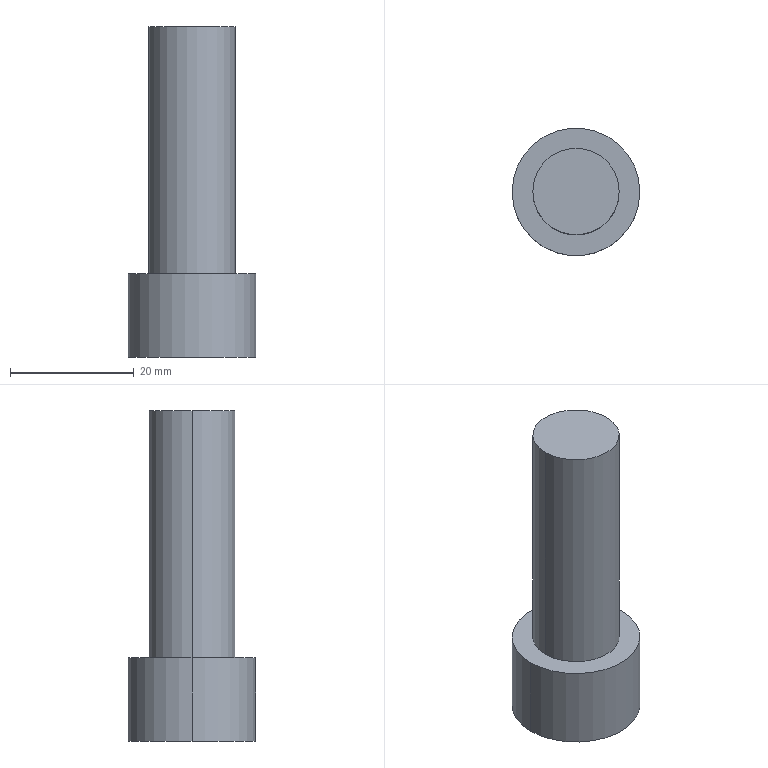Part | STEP file | M14 screw | 1 solid | 7 faces | box 20.67 x 20.67 x 53.57 mm | volume 10711 mm3 | cylinder 4 | plane 3 | commonest cylinder face diameters 14 x2 20.67 x2
STEP:
#1=CARTESIAN_POINT('',(0.,0.,0.));
#2=DIRECTION('',(0.,0.,1.));
#3=DIRECTION('',(1.,0.,0.));
#4=AXIS2_PLACEMENT_3D('',#1,#2,#3);
#5=CARTESIAN_POINT('',(7.,0.,53.57));
#6=VERTEX_POINT('',#5);
#7=CARTESIAN_POINT('',(-7.,0.,53.57));
#8=VERTEX_POINT('',#7);
#9=CARTESIAN_POINT('',(0.,0.,53.57));
#10=DIRECTION('',(0.,0.,1.));
#11=DIRECTION('',(1.,0.,0.));
#12=AXIS2_PLACEMENT_3D('',#9,#10,#11);
#13=CIRCLE('',#12,7.);
#14=CARTESIAN_POINT('',(0.,0.,53.57));
#15=DIRECTION('',(0.,0.,-1.));
#16=DIRECTION('',(-1.,0.,0.));
#17=AXIS2_PLACEMENT_3D('',#14,#15,#16);
#18=CYLINDRICAL_SURFACE('',#17,7.);
#19=CARTESIAN_POINT('',(3.142,0.));
#20=DIRECTION('',(-1.,0.));
#21=VECTOR('',#20,1.);
#22=LINE('',#19,#21);
#23=(GEOMETRIC_REPRESENTATION_CONTEXT(2)PARAMETRIC_REPRESENTATION_CONTEXT()REPRESENTATION_CONTEXT('',''));
#24=DEFINITIONAL_REPRESENTATION('',(#22),#23);
#25=PCURVE('',#18,#24);
#26=CARTESIAN_POINT('',(0.,0.,53.57));
#27=DIRECTION('',(0.,0.,1.));
#28=DIRECTION('',(1.,0.,0.));
#29=AXIS2_PLACEMENT_3D('',#26,#27,#28);
#30=PLANE('',#29);
#31=CARTESIAN_POINT('',(0.,0.));
#32=DIRECTION('',(1.,0.));
#33=AXIS2_PLACEMENT_2D('',#31,#32);
#34=CIRCLE('',#33,7.);
#35=(GEOMETRIC_REPRESENTATION_CONTEXT(2)PARAMETRIC_REPRESENTATION_CONTEXT()REPRESENTATION_CONTEXT('',''));
#36=DEFINITIONAL_REPRESENTATION('',(#34),#35);
#37=PCURVE('',#30,#36);
#38=SURFACE_CURVE('',#13,(#25,#37),.PCURVE_S1.);
#39=EDGE_CURVE('',#6,#8,#38,.T.);
#40=ORIENTED_EDGE('',*,*,#39,.F.);
#41=CARTESIAN_POINT('',(7.,0.,13.57));
#42=VERTEX_POINT('',#41);
#43=CARTESIAN_POINT('',(7.,0.,53.57));
#44=DIRECTION('',(0.,0.,-1.));
#45=VECTOR('',#44,1.);
#46=LINE('',#43,#45);
#47=CARTESIAN_POINT('',(3.142,0.));
#48=DIRECTION('',(0.,1.));
#49=VECTOR('',#48,1.);
#50=LINE('',#47,#49);
#51=(GEOMETRIC_REPRESENTATION_CONTEXT(2)PARAMETRIC_REPRESENTATION_CONTEXT()REPRESENTATION_CONTEXT('',''));
#52=DEFINITIONAL_REPRESENTATION('',(#50),#51);
#53=PCURVE('',#18,#52);
#54=CARTESIAN_POINT('',(0.,0.,53.57));
#55=DIRECTION('',(0.,0.,-1.));
#56=DIRECTION('',(-1.,0.,0.));
#57=AXIS2_PLACEMENT_3D('',#54,#55,#56);
#58=CYLINDRICAL_SURFACE('',#57,7.);
#59=CARTESIAN_POINT('',(3.142,0.));
#60=DIRECTION('',(0.,1.));
#61=VECTOR('',#60,1.);
#62=LINE('',#59,#61);
#63=(GEOMETRIC_REPRESENTATION_CONTEXT(2)PARAMETRIC_REPRESENTATION_CONTEXT()REPRESENTATION_CONTEXT('',''));
#64=DEFINITIONAL_REPRESENTATION('',(#62),#63);
#65=PCURVE('',#58,#64);
#66=SURFACE_CURVE('',#46,(#53,#65),.PCURVE_S1.);
#67=EDGE_CURVE('',#6,#42,#66,.T.);
#68=ORIENTED_EDGE('',*,*,#67,.T.);
#69=CARTESIAN_POINT('',(-7.,0.,13.57));
#70=VERTEX_POINT('',#69);
#71=CARTESIAN_POINT('',(0.,0.,13.57));
#72=DIRECTION('',(0.,0.,1.));
#73=DIRECTION('',(1.,0.,0.));
#74=AXIS2_PLACEMENT_3D('',#71,#72,#73);
#75=CIRCLE('',#74,7.);
#76=CARTESIAN_POINT('',(3.142,40.));
#77=DIRECTION('',(-1.,0.));
#78=VECTOR('',#77,1.);
#79=LINE('',#76,#78);
#80=(GEOMETRIC_REPRESENTATION_CONTEXT(2)PARAMETRIC_REPRESENTATION_CONTEXT()REPRESENTATION_CONTEXT('',''));
#81=DEFINITIONAL_REPRESENTATION('',(#79),#80);
#82=PCURVE('',#18,#81);
#83=CARTESIAN_POINT('',(0.,0.,13.57));
#84=DIRECTION('',(0.,0.,1.));
#85=DIRECTION('',(1.,0.,0.));
#86=AXIS2_PLACEMENT_3D('',#83,#84,#85);
#87=PLANE('',#86);
#88=CARTESIAN_POINT('',(0.,0.));
#89=DIRECTION('',(1.,0.));
#90=AXIS2_PLACEMENT_2D('',#88,#89);
#91=CIRCLE('',#90,7.);
#92=(GEOMETRIC_REPRESENTATION_CONTEXT(2)PARAMETRIC_REPRESENTATION_CONTEXT()REPRESENTATION_CONTEXT('',''));
#93=DEFINITIONAL_REPRESENTATION('',(#91),#92);
#94=PCURVE('',#87,#93);
#95=SURFACE_CURVE('',#75,(#82,#94),.PCURVE_S1.);
#96=EDGE_CURVE('',#42,#70,#95,.T.);
#97=ORIENTED_EDGE('',*,*,#96,.T.);
#98=CARTESIAN_POINT('',(-7.,0.,53.57));
#99=DIRECTION('',(0.,0.,-1.));
#100=VECTOR('',#99,1.);
#101=LINE('',#98,#100);
#102=CARTESIAN_POINT('',(0.,0.));
#103=DIRECTION('',(0.,1.));
#104=VECTOR('',#103,1.);
#105=LINE('',#102,#104);
#106=(GEOMETRIC_REPRESENTATION_CONTEXT(2)PARAMETRIC_REPRESENTATION_CONTEXT()REPRESENTATION_CONTEXT('',''));
#107=DEFINITIONAL_REPRESENTATION('',(#105),#106);
#108=PCURVE('',#18,#107);
#109=CARTESIAN_POINT('',(6.283,0.));
#110=DIRECTION('',(0.,1.));
#111=VECTOR('',#110,1.);
#112=LINE('',#109,#111);
#113=(GEOMETRIC_REPRESENTATION_CONTEXT(2)PARAMETRIC_REPRESENTATION_CONTEXT()REPRESENTATION_CONTEXT('',''));
#114=DEFINITIONAL_REPRESENTATION('',(#112),#113);
#115=PCURVE('',#58,#114);
#116=SURFACE_CURVE('',#101,(#108,#115),.PCURVE_S1.);
#117=EDGE_CURVE('',#8,#70,#116,.T.);
#118=ORIENTED_EDGE('',*,*,#117,.F.);
#119=EDGE_LOOP('',(#40,#68,#97,#118));
#120=FACE_BOUND('',#119,.T.);
#121=ADVANCED_FACE('',(#120),#18,.T.);
#122=CARTESIAN_POINT('',(10.335,0.,13.57));
#123=VERTEX_POINT('',#122);
#124=CARTESIAN_POINT('',(-10.335,0.,13.57));
#125=VERTEX_POINT('',#124);
#126=CARTESIAN_POINT('',(0.,0.,13.57));
#127=DIRECTION('',(0.,0.,1.));
#128=DIRECTION('',(1.,0.,0.));
#129=AXIS2_PLACEMENT_3D('',#126,#127,#128);
#130=CIRCLE('',#129,10.335);
#131=CARTESIAN_POINT('',(0.,0.,13.57));
#132=DIRECTION('',(0.,0.,-1.));
#133=DIRECTION('',(-1.,0.,0.));
#134=AXIS2_PLACEMENT_3D('',#131,#132,#133);
#135=CYLINDRICAL_SURFACE('',#134,10.335);
#136=CARTESIAN_POINT('',(3.142,0.));
#137=DIRECTION('',(-1.,0.));
#138=VECTOR('',#137,1.);
#139=LINE('',#136,#138);
#140=(GEOMETRIC_REPRESENTATION_CONTEXT(2)PARAMETRIC_REPRESENTATION_CONTEXT()REPRESENTATION_CONTEXT('',''));
#141=DEFINITIONAL_REPRESENTATION('',(#139),#140);
#142=PCURVE('',#135,#141);
#143=CARTESIAN_POINT('',(0.,0.));
#144=DIRECTION('',(1.,0.));
#145=AXIS2_PLACEMENT_2D('',#143,#144);
#146=CIRCLE('',#145,10.335);
#147=(GEOMETRIC_REPRESENTATION_CONTEXT(2)PARAMETRIC_REPRESENTATION_CONTEXT()REPRESENTATION_CONTEXT('',''));
#148=DEFINITIONAL_REPRESENTATION('',(#146),#147);
#149=PCURVE('',#87,#148);
#150=SURFACE_CURVE('',#130,(#142,#149),.PCURVE_S1.);
#151=EDGE_CURVE('',#123,#125,#150,.T.);
#152=ORIENTED_EDGE('',*,*,#151,.F.);
#153=CARTESIAN_POINT('',(10.335,0.,0.));
#154=VERTEX_POINT('',#153);
#155=CARTESIAN_POINT('',(10.335,0.,13.57));
#156=DIRECTION('',(0.,0.,-1.));
#157=VECTOR('',#156,1.);
#158=LINE('',#155,#157);
#159=CARTESIAN_POINT('',(3.142,0.));
#160=DIRECTION('',(0.,1.));
#161=VECTOR('',#160,1.);
#162=LINE('',#159,#161);
#163=(GEOMETRIC_REPRESENTATION_CONTEXT(2)PARAMETRIC_REPRESENTATION_CONTEXT()REPRESENTATION_CONTEXT('',''));
#164=DEFINITIONAL_REPRESENTATION('',(#162),#163);
#165=PCURVE('',#135,#164);
#166=CARTESIAN_POINT('',(0.,0.,13.57));
#167=DIRECTION('',(0.,0.,-1.));
#168=DIRECTION('',(-1.,0.,0.));
#169=AXIS2_PLACEMENT_3D('',#166,#167,#168);
#170=CYLINDRICAL_SURFACE('',#169,10.335);
#171=CARTESIAN_POINT('',(3.142,0.));
#172=DIRECTION('',(0.,1.));
#173=VECTOR('',#172,1.);
#174=LINE('',#171,#173);
#175=(GEOMETRIC_REPRESENTATION_CONTEXT(2)PARAMETRIC_REPRESENTATION_CONTEXT()REPRESENTATION_CONTEXT('',''));
#176=DEFINITIONAL_REPRESENTATION('',(#174),#175);
#177=PCURVE('',#170,#176);
#178=SURFACE_CURVE('',#158,(#165,#177),.PCURVE_S1.);
#179=EDGE_CURVE('',#123,#154,#178,.T.);
#180=ORIENTED_EDGE('',*,*,#179,.T.);
#181=CARTESIAN_POINT('',(-10.335,0.,0.));
#182=VERTEX_POINT('',#181);
#183=CARTESIAN_POINT('',(0.,0.,0.));
#184=DIRECTION('',(0.,0.,1.));
#185=DIRECTION('',(1.,0.,0.));
#186=AXIS2_PLACEMENT_3D('',#183,#184,#185);
#187=CIRCLE('',#186,10.335);
#188=CARTESIAN_POINT('',(3.142,13.57));
#189=DIRECTION('',(-1.,0.));
#190=VECTOR('',#189,1.);
#191=LINE('',#188,#190);
#192=(GEOMETRIC_REPRESENTATION_CONTEXT(2)PARAMETRIC_REPRESENTATION_CONTEXT()REPRESENTATION_CONTEXT('',''));
#193=DEFINITIONAL_REPRESENTATION('',(#191),#192);
#194=PCURVE('',#135,#193);
#195=CARTESIAN_POINT('',(0.,0.,0.));
#196=DIRECTION('',(0.,0.,1.));
#197=DIRECTION('',(1.,0.,0.));
#198=AXIS2_PLACEMENT_3D('',#195,#196,#197);
#199=PLANE('',#198);
#200=CARTESIAN_POINT('',(0.,0.));
#201=DIRECTION('',(1.,0.));
#202=AXIS2_PLACEMENT_2D('',#200,#201);
#203=CIRCLE('',#202,10.335);
#204=(GEOMETRIC_REPRESENTATION_CONTEXT(2)PARAMETRIC_REPRESENTATION_CONTEXT()REPRESENTATION_CONTEXT('',''));
#205=DEFINITIONAL_REPRESENTATION('',(#203),#204);
#206=PCURVE('',#199,#205);
#207=SURFACE_CURVE('',#187,(#194,#206),.PCURVE_S1.);
#208=EDGE_CURVE('',#154,#182,#207,.T.);
#209=ORIENTED_EDGE('',*,*,#208,.T.);
#210=CARTESIAN_POINT('',(-10.335,0.,13.57));
#211=DIRECTION('',(0.,0.,-1.));
#212=VECTOR('',#211,1.);
#213=LINE('',#210,#212);
#214=CARTESIAN_POINT('',(0.,0.));
#215=DIRECTION('',(0.,1.));
#216=VECTOR('',#215,1.);
#217=LINE('',#214,#216);
#218=(GEOMETRIC_REPRESENTATION_CONTEXT(2)PARAMETRIC_REPRESENTATION_CONTEXT()REPRESENTATION_CONTEXT('',''));
#219=DEFINITIONAL_REPRESENTATION('',(#217),#218);
#220=PCURVE('',#135,#219);
#221=CARTESIAN_POINT('',(6.283,0.));
#222=DIRECTION('',(0.,1.));
#223=VECTOR('',#222,1.);
#224=LINE('',#221,#223);
#225=(GEOMETRIC_REPRESENTATION_CONTEXT(2)PARAMETRIC_REPRESENTATION_CONTEXT()REPRESENTATION_CONTEXT('',''));
#226=DEFINITIONAL_REPRESENTATION('',(#224),#225);
#227=PCURVE('',#170,#226);
#228=SURFACE_CURVE('',#213,(#220,#227),.PCURVE_S1.);
#229=EDGE_CURVE('',#125,#182,#228,.T.);
#230=ORIENTED_EDGE('',*,*,#229,.F.);
#231=EDGE_LOOP('',(#152,#180,#209,#230));
#232=FACE_BOUND('',#231,.T.);
#233=ADVANCED_FACE('',(#232),#135,.T.);
#234=CARTESIAN_POINT('',(0.,0.,13.57));
#235=DIRECTION('',(0.,0.,1.));
#236=DIRECTION('',(1.,0.,0.));
#237=AXIS2_PLACEMENT_3D('',#234,#235,#236);
#238=CIRCLE('',#237,10.335);
#239=CARTESIAN_POINT('',(0.,0.));
#240=DIRECTION('',(1.,0.));
#241=AXIS2_PLACEMENT_2D('',#239,#240);
#242=CIRCLE('',#241,10.335);
#243=(GEOMETRIC_REPRESENTATION_CONTEXT(2)PARAMETRIC_REPRESENTATION_CONTEXT()REPRESENTATION_CONTEXT('',''));
#244=DEFINITIONAL_REPRESENTATION('',(#242),#243);
#245=PCURVE('',#87,#244);
#246=CARTESIAN_POINT('',(9.425,0.));
#247=DIRECTION('',(-1.,0.));
#248=VECTOR('',#247,1.);
#249=LINE('',#246,#248);
#250=(GEOMETRIC_REPRESENTATION_CONTEXT(2)PARAMETRIC_REPRESENTATION_CONTEXT()REPRESENTATION_CONTEXT('',''));
#251=DEFINITIONAL_REPRESENTATION('',(#249),#250);
#252=PCURVE('',#170,#251);
#253=SURFACE_CURVE('',#238,(#245,#252),.PCURVE_S1.);
#254=EDGE_CURVE('',#125,#123,#253,.T.);
#255=ORIENTED_EDGE('',*,*,#254,.T.);
#256=ORIENTED_EDGE('',*,*,#151,.T.);
#257=EDGE_LOOP('',(#255,#256));
#258=FACE_BOUND('',#257,.T.);
#259=CARTESIAN_POINT('',(0.,0.,13.57));
#260=DIRECTION('',(0.,0.,1.));
#261=DIRECTION('',(1.,0.,0.));
#262=AXIS2_PLACEMENT_3D('',#259,#260,#261);
#263=CIRCLE('',#262,7.);
#264=CARTESIAN_POINT('',(0.,0.));
#265=DIRECTION('',(1.,0.));
#266=AXIS2_PLACEMENT_2D('',#264,#265);
#267=CIRCLE('',#266,7.);
#268=(GEOMETRIC_REPRESENTATION_CONTEXT(2)PARAMETRIC_REPRESENTATION_CONTEXT()REPRESENTATION_CONTEXT('',''));
#269=DEFINITIONAL_REPRESENTATION('',(#267),#268);
#270=PCURVE('',#87,#269);
#271=CARTESIAN_POINT('',(9.425,40.));
#272=DIRECTION('',(-1.,0.));
#273=VECTOR('',#272,1.);
#274=LINE('',#271,#273);
#275=(GEOMETRIC_REPRESENTATION_CONTEXT(2)PARAMETRIC_REPRESENTATION_CONTEXT()REPRESENTATION_CONTEXT('',''));
#276=DEFINITIONAL_REPRESENTATION('',(#274),#275);
#277=PCURVE('',#58,#276);
#278=SURFACE_CURVE('',#263,(#270,#277),.PCURVE_S1.);
#279=EDGE_CURVE('',#70,#42,#278,.T.);
#280=ORIENTED_EDGE('',*,*,#279,.F.);
#281=ORIENTED_EDGE('',*,*,#96,.F.);
#282=EDGE_LOOP('',(#280,#281));
#283=FACE_BOUND('',#282,.T.);
#284=ADVANCED_FACE('',(#258,#283),#87,.T.);
#285=ORIENTED_EDGE('',*,*,#179,.F.);
#286=ORIENTED_EDGE('',*,*,#254,.F.);
#287=ORIENTED_EDGE('',*,*,#229,.T.);
#288=CARTESIAN_POINT('',(0.,0.,0.));
#289=DIRECTION('',(0.,0.,1.));
#290=DIRECTION('',(1.,0.,0.));
#291=AXIS2_PLACEMENT_3D('',#288,#289,#290);
#292=CIRCLE('',#291,10.335);
#293=CARTESIAN_POINT('',(9.425,13.57));
#294=DIRECTION('',(-1.,0.));
#295=VECTOR('',#294,1.);
#296=LINE('',#293,#295);
#297=(GEOMETRIC_REPRESENTATION_CONTEXT(2)PARAMETRIC_REPRESENTATION_CONTEXT()REPRESENTATION_CONTEXT('',''));
#298=DEFINITIONAL_REPRESENTATION('',(#296),#297);
#299=PCURVE('',#170,#298);
#300=CARTESIAN_POINT('',(0.,0.));
#301=DIRECTION('',(1.,0.));
#302=AXIS2_PLACEMENT_2D('',#300,#301);
#303=CIRCLE('',#302,10.335);
#304=(GEOMETRIC_REPRESENTATION_CONTEXT(2)PARAMETRIC_REPRESENTATION_CONTEXT()REPRESENTATION_CONTEXT('',''));
#305=DEFINITIONAL_REPRESENTATION('',(#303),#304);
#306=PCURVE('',#199,#305);
#307=SURFACE_CURVE('',#292,(#299,#306),.PCURVE_S1.);
#308=EDGE_CURVE('',#182,#154,#307,.T.);
#309=ORIENTED_EDGE('',*,*,#308,.T.);
#310=EDGE_LOOP('',(#285,#286,#287,#309));
#311=FACE_BOUND('',#310,.T.);
#312=ADVANCED_FACE('',(#311),#170,.T.);
#313=ORIENTED_EDGE('',*,*,#308,.F.);
#314=ORIENTED_EDGE('',*,*,#208,.F.);
#315=EDGE_LOOP('',(#313,#314));
#316=FACE_BOUND('',#315,.T.);
#317=ADVANCED_FACE('',(#316),#199,.F.);
#318=ORIENTED_EDGE('',*,*,#67,.F.);
#319=CARTESIAN_POINT('',(0.,0.,53.57));
#320=DIRECTION('',(0.,0.,1.));
#321=DIRECTION('',(1.,0.,0.));
#322=AXIS2_PLACEMENT_3D('',#319,#320,#321);
#323=CIRCLE('',#322,7.);
#324=CARTESIAN_POINT('',(9.425,0.));
#325=DIRECTION('',(-1.,0.));
#326=VECTOR('',#325,1.);
#327=LINE('',#324,#326);
#328=(GEOMETRIC_REPRESENTATION_CONTEXT(2)PARAMETRIC_REPRESENTATION_CONTEXT()REPRESENTATION_CONTEXT('',''));
#329=DEFINITIONAL_REPRESENTATION('',(#327),#328);
#330=PCURVE('',#58,#329);
#331=CARTESIAN_POINT('',(0.,0.));
#332=DIRECTION('',(1.,0.));
#333=AXIS2_PLACEMENT_2D('',#331,#332);
#334=CIRCLE('',#333,7.);
#335=(GEOMETRIC_REPRESENTATION_CONTEXT(2)PARAMETRIC_REPRESENTATION_CONTEXT()REPRESENTATION_CONTEXT('',''));
#336=DEFINITIONAL_REPRESENTATION('',(#334),#335);
#337=PCURVE('',#30,#336);
#338=SURFACE_CURVE('',#323,(#330,#337),.PCURVE_S1.);
#339=EDGE_CURVE('',#8,#6,#338,.T.);
#340=ORIENTED_EDGE('',*,*,#339,.F.);
#341=ORIENTED_EDGE('',*,*,#117,.T.);
#342=ORIENTED_EDGE('',*,*,#279,.T.);
#343=EDGE_LOOP('',(#318,#340,#341,#342));
#344=FACE_BOUND('',#343,.T.);
#345=ADVANCED_FACE('',(#344),#58,.T.);
#346=ORIENTED_EDGE('',*,*,#339,.T.);
#347=ORIENTED_EDGE('',*,*,#39,.T.);
#348=EDGE_LOOP('',(#346,#347));
#349=FACE_BOUND('',#348,.T.);
#350=ADVANCED_FACE('',(#349),#30,.T.);
#351=CLOSED_SHELL('',(#121,#233,#284,#312,#317,#345,#350));
#352=MANIFOLD_SOLID_BREP('',#351);
#353=(LENGTH_UNIT()NAMED_UNIT(*)SI_UNIT(.MILLI.,.METRE.));
#354=UNCERTAINTY_MEASURE_WITH_UNIT(LENGTH_MEASURE(0.0000001),#353,'','');
#355=(NAMED_UNIT(*)PLANE_ANGLE_UNIT()SI_UNIT($,.RADIAN.));
#356=(NAMED_UNIT(*)SI_UNIT($,.STERADIAN.)SOLID_ANGLE_UNIT());
#357=(GEOMETRIC_REPRESENTATION_CONTEXT(3)GLOBAL_UNCERTAINTY_ASSIGNED_CONTEXT((#354))GLOBAL_UNIT_ASSIGNED_CONTEXT((#353,#355,#356))REPRESENTATION_CONTEXT('',''));
#358=ADVANCED_BREP_SHAPE_REPRESENTATION('',(#4,#352),#357);